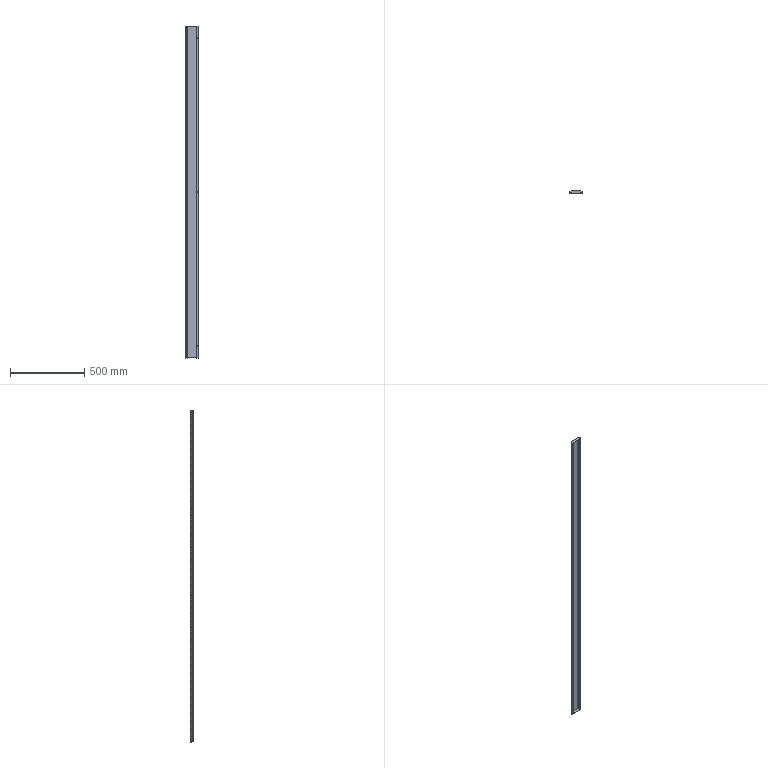Part | STEP file | Front Trim Panel | 1 solid | 86 faces | box 85 x 20 x 2241 mm | volume 442724 mm3 | plane 54 | cylinder 32 | commonest cylinder face diameters 3.2 x12 1 x11 4 x8 0.944 x1